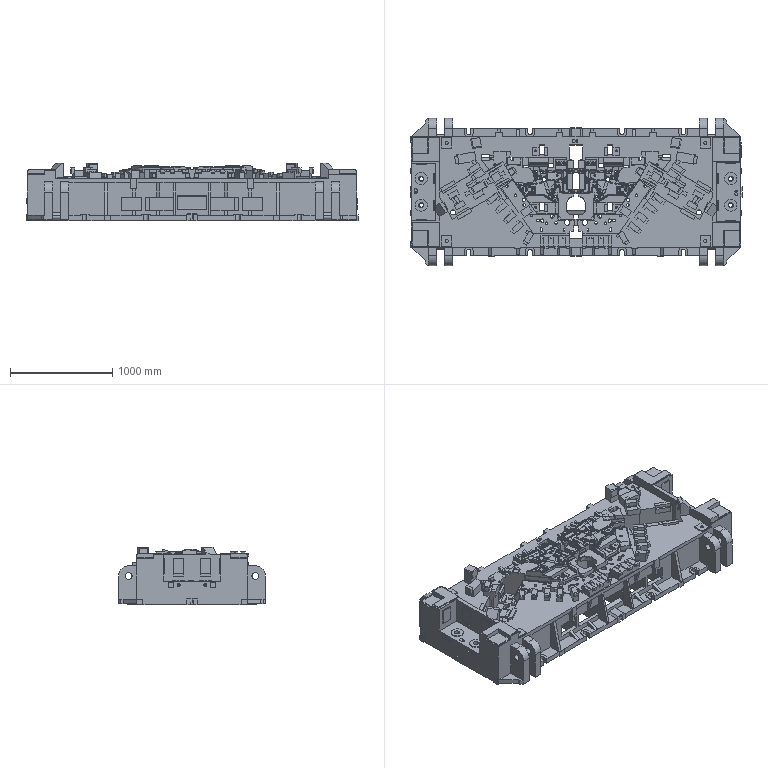Part | NX | features solid 2 | 1 solid | 3667 faces | volume 642512787 mm3 | plane 2133 | spline 1316 | cylinder 216 | sphere 2 | commonest cylinder face diameters 50 x27 25 x26 20 x25 30 x18 68 x16 28 x12